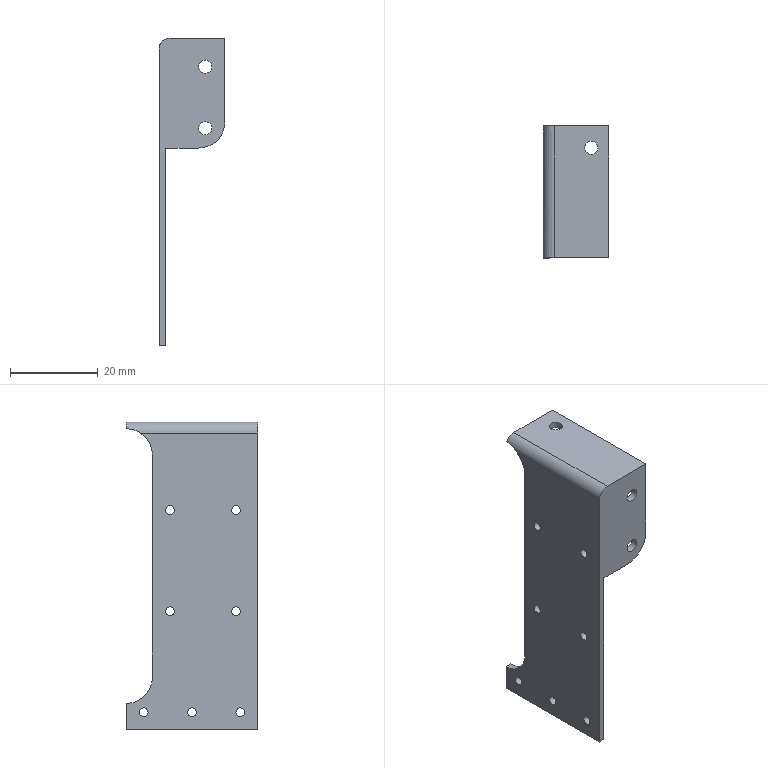Part | STEP file | 1-47.1 | 1 solid | 27 faces | box 15 x 30 x 70 mm | volume 3583 mm3 | cylinder 13 | plane 12 | spline 2 | commonest cylinder face diameters 2 x7 3 x3 12 x2 5 x1